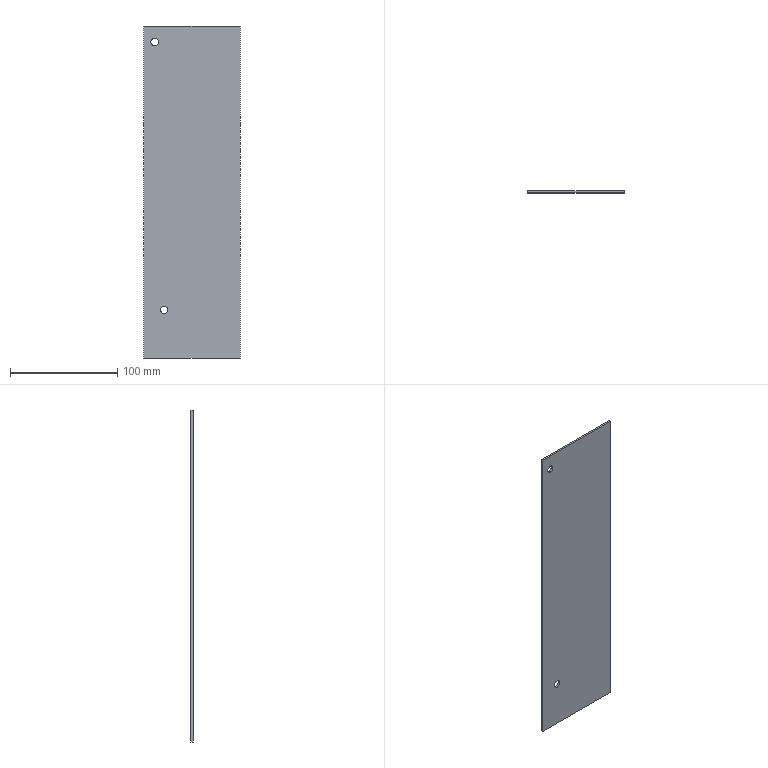Part | STEP file | Bottom plate secondary wiring hole cover | 1 solid | 10 faces | box 90 x 2 x 310 mm | volume 55646 mm3 | plane 6 | cylinder 4 | commonest cylinder face diameters 7 x4
STEP:
#1=CARTESIAN_POINT('',(0.,0.,0.));
#2=DIRECTION('',(0.,0.,1.));
#3=DIRECTION('',(1.,0.,0.));
#4=AXIS2_PLACEMENT_3D('',#1,#2,#3);
#5=CARTESIAN_POINT('',(10.,-2.,-11.5));
#6=VERTEX_POINT('',#5);
#7=CARTESIAN_POINT('',(10.,0.,-11.5));
#8=VERTEX_POINT('',#7);
#9=CARTESIAN_POINT('',(10.,-10.,-11.5));
#10=DIRECTION('',(0.,1.,0.));
#11=VECTOR('',#10,1.);
#12=LINE('',#9,#11);
#13=CARTESIAN_POINT('',(10.,-10.,-15.));
#14=DIRECTION('',(0.,1.,0.));
#15=DIRECTION('',(0.,0.,1.));
#16=AXIS2_PLACEMENT_3D('',#13,#14,#15);
#17=CYLINDRICAL_SURFACE('',#16,3.5);
#18=CARTESIAN_POINT('',(6.283,0.));
#19=DIRECTION('',(0.,1.));
#20=VECTOR('',#19,1.);
#21=LINE('',#18,#20);
#22=(GEOMETRIC_REPRESENTATION_CONTEXT(2)PARAMETRIC_REPRESENTATION_CONTEXT()REPRESENTATION_CONTEXT('',''));
#23=DEFINITIONAL_REPRESENTATION('',(#21),#22);
#24=PCURVE('',#17,#23);
#25=CARTESIAN_POINT('',(10.,-10.,-15.));
#26=DIRECTION('',(0.,1.,0.));
#27=DIRECTION('',(0.,0.,1.));
#28=AXIS2_PLACEMENT_3D('',#25,#26,#27);
#29=CYLINDRICAL_SURFACE('',#28,3.5);
#30=CARTESIAN_POINT('',(0.,0.));
#31=DIRECTION('',(0.,1.));
#32=VECTOR('',#31,1.);
#33=LINE('',#30,#32);
#34=(GEOMETRIC_REPRESENTATION_CONTEXT(2)PARAMETRIC_REPRESENTATION_CONTEXT()REPRESENTATION_CONTEXT('',''));
#35=DEFINITIONAL_REPRESENTATION('',(#33),#34);
#36=PCURVE('',#29,#35);
#37=SURFACE_CURVE('',#12,(#24,#36),.PCURVE_S1.);
#38=EDGE_CURVE('',#6,#8,#37,.T.);
#39=ORIENTED_EDGE('',*,*,#38,.T.);
#40=CARTESIAN_POINT('',(10.,0.,-18.5));
#41=VERTEX_POINT('',#40);
#42=CARTESIAN_POINT('',(10.,0.,-15.));
#43=DIRECTION('',(0.,1.,0.));
#44=DIRECTION('',(0.,0.,1.));
#45=AXIS2_PLACEMENT_3D('',#42,#43,#44);
#46=CIRCLE('',#45,3.5);
#47=CARTESIAN_POINT('',(0.,10.));
#48=DIRECTION('',(1.,0.));
#49=VECTOR('',#48,1.);
#50=LINE('',#47,#49);
#51=(GEOMETRIC_REPRESENTATION_CONTEXT(2)PARAMETRIC_REPRESENTATION_CONTEXT()REPRESENTATION_CONTEXT('',''));
#52=DEFINITIONAL_REPRESENTATION('',(#50),#51);
#53=PCURVE('',#17,#52);
#54=CARTESIAN_POINT('',(0.,0.,0.));
#55=DIRECTION('',(0.,1.,0.));
#56=DIRECTION('',(0.,0.,1.));
#57=AXIS2_PLACEMENT_3D('',#54,#55,#56);
#58=PLANE('',#57);
#59=CARTESIAN_POINT('',(-15.,10.));
#60=DIRECTION('',(1.,0.));
#61=AXIS2_PLACEMENT_2D('',#59,#60);
#62=CIRCLE('',#61,3.5);
#63=(GEOMETRIC_REPRESENTATION_CONTEXT(2)PARAMETRIC_REPRESENTATION_CONTEXT()REPRESENTATION_CONTEXT('',''));
#64=DEFINITIONAL_REPRESENTATION('',(#62),#63);
#65=PCURVE('',#58,#64);
#66=SURFACE_CURVE('',#46,(#53,#65),.PCURVE_S1.);
#67=EDGE_CURVE('',#41,#8,#66,.T.);
#68=ORIENTED_EDGE('',*,*,#67,.F.);
#69=CARTESIAN_POINT('',(10.,-2.,-18.5));
#70=VERTEX_POINT('',#69);
#71=CARTESIAN_POINT('',(10.,-10.,-18.5));
#72=DIRECTION('',(0.,1.,0.));
#73=VECTOR('',#72,1.);
#74=LINE('',#71,#73);
#75=CARTESIAN_POINT('',(3.142,0.));
#76=DIRECTION('',(0.,1.));
#77=VECTOR('',#76,1.);
#78=LINE('',#75,#77);
#79=(GEOMETRIC_REPRESENTATION_CONTEXT(2)PARAMETRIC_REPRESENTATION_CONTEXT()REPRESENTATION_CONTEXT('',''));
#80=DEFINITIONAL_REPRESENTATION('',(#78),#79);
#81=PCURVE('',#17,#80);
#82=CARTESIAN_POINT('',(3.142,0.));
#83=DIRECTION('',(0.,1.));
#84=VECTOR('',#83,1.);
#85=LINE('',#82,#84);
#86=(GEOMETRIC_REPRESENTATION_CONTEXT(2)PARAMETRIC_REPRESENTATION_CONTEXT()REPRESENTATION_CONTEXT('',''));
#87=DEFINITIONAL_REPRESENTATION('',(#85),#86);
#88=PCURVE('',#29,#87);
#89=SURFACE_CURVE('',#74,(#81,#88),.PCURVE_S1.);
#90=EDGE_CURVE('',#70,#41,#89,.T.);
#91=ORIENTED_EDGE('',*,*,#90,.F.);
#92=CARTESIAN_POINT('',(10.,-2.,-15.));
#93=DIRECTION('',(0.,1.,0.));
#94=DIRECTION('',(0.,0.,1.));
#95=AXIS2_PLACEMENT_3D('',#92,#93,#94);
#96=CIRCLE('',#95,3.5);
#97=CARTESIAN_POINT('',(0.,8.));
#98=DIRECTION('',(1.,0.));
#99=VECTOR('',#98,1.);
#100=LINE('',#97,#99);
#101=(GEOMETRIC_REPRESENTATION_CONTEXT(2)PARAMETRIC_REPRESENTATION_CONTEXT()REPRESENTATION_CONTEXT('',''));
#102=DEFINITIONAL_REPRESENTATION('',(#100),#101);
#103=PCURVE('',#17,#102);
#104=CARTESIAN_POINT('',(0.,-2.,0.));
#105=DIRECTION('',(0.,1.,0.));
#106=DIRECTION('',(0.,0.,1.));
#107=AXIS2_PLACEMENT_3D('',#104,#105,#106);
#108=PLANE('',#107);
#109=CARTESIAN_POINT('',(-15.,10.));
#110=DIRECTION('',(1.,0.));
#111=AXIS2_PLACEMENT_2D('',#109,#110);
#112=CIRCLE('',#111,3.5);
#113=(GEOMETRIC_REPRESENTATION_CONTEXT(2)PARAMETRIC_REPRESENTATION_CONTEXT()REPRESENTATION_CONTEXT('',''));
#114=DEFINITIONAL_REPRESENTATION('',(#112),#113);
#115=PCURVE('',#108,#114);
#116=SURFACE_CURVE('',#96,(#103,#115),.PCURVE_S1.);
#117=EDGE_CURVE('',#70,#6,#116,.T.);
#118=ORIENTED_EDGE('',*,*,#117,.T.);
#119=EDGE_LOOP('',(#39,#68,#91,#118));
#120=FACE_BOUND('',#119,.F.);
#121=ADVANCED_FACE('',(#120),#17,.F.);
#122=CARTESIAN_POINT('',(19.,-2.,-261.5));
#123=VERTEX_POINT('',#122);
#124=CARTESIAN_POINT('',(19.,0.,-261.5));
#125=VERTEX_POINT('',#124);
#126=CARTESIAN_POINT('',(19.,-10.,-261.5));
#127=DIRECTION('',(0.,1.,0.));
#128=VECTOR('',#127,1.);
#129=LINE('',#126,#128);
#130=CARTESIAN_POINT('',(19.,-10.,-265.));
#131=DIRECTION('',(0.,1.,0.));
#132=DIRECTION('',(0.,0.,1.));
#133=AXIS2_PLACEMENT_3D('',#130,#131,#132);
#134=CYLINDRICAL_SURFACE('',#133,3.5);
#135=CARTESIAN_POINT('',(6.283,0.));
#136=DIRECTION('',(0.,1.));
#137=VECTOR('',#136,1.);
#138=LINE('',#135,#137);
#139=(GEOMETRIC_REPRESENTATION_CONTEXT(2)PARAMETRIC_REPRESENTATION_CONTEXT()REPRESENTATION_CONTEXT('',''));
#140=DEFINITIONAL_REPRESENTATION('',(#138),#139);
#141=PCURVE('',#134,#140);
#142=CARTESIAN_POINT('',(19.,-10.,-265.));
#143=DIRECTION('',(0.,1.,0.));
#144=DIRECTION('',(0.,0.,1.));
#145=AXIS2_PLACEMENT_3D('',#142,#143,#144);
#146=CYLINDRICAL_SURFACE('',#145,3.5);
#147=CARTESIAN_POINT('',(0.,0.));
#148=DIRECTION('',(0.,1.));
#149=VECTOR('',#148,1.);
#150=LINE('',#147,#149);
#151=(GEOMETRIC_REPRESENTATION_CONTEXT(2)PARAMETRIC_REPRESENTATION_CONTEXT()REPRESENTATION_CONTEXT('',''));
#152=DEFINITIONAL_REPRESENTATION('',(#150),#151);
#153=PCURVE('',#146,#152);
#154=SURFACE_CURVE('',#129,(#141,#153),.PCURVE_S1.);
#155=EDGE_CURVE('',#123,#125,#154,.T.);
#156=ORIENTED_EDGE('',*,*,#155,.T.);
#157=CARTESIAN_POINT('',(19.,0.,-268.5));
#158=VERTEX_POINT('',#157);
#159=CARTESIAN_POINT('',(19.,0.,-265.));
#160=DIRECTION('',(0.,1.,0.));
#161=DIRECTION('',(0.,0.,1.));
#162=AXIS2_PLACEMENT_3D('',#159,#160,#161);
#163=CIRCLE('',#162,3.5);
#164=CARTESIAN_POINT('',(0.,10.));
#165=DIRECTION('',(1.,0.));
#166=VECTOR('',#165,1.);
#167=LINE('',#164,#166);
#168=(GEOMETRIC_REPRESENTATION_CONTEXT(2)PARAMETRIC_REPRESENTATION_CONTEXT()REPRESENTATION_CONTEXT('',''));
#169=DEFINITIONAL_REPRESENTATION('',(#167),#168);
#170=PCURVE('',#134,#169);
#171=CARTESIAN_POINT('',(-265.,19.));
#172=DIRECTION('',(1.,0.));
#173=AXIS2_PLACEMENT_2D('',#171,#172);
#174=CIRCLE('',#173,3.5);
#175=(GEOMETRIC_REPRESENTATION_CONTEXT(2)PARAMETRIC_REPRESENTATION_CONTEXT()REPRESENTATION_CONTEXT('',''));
#176=DEFINITIONAL_REPRESENTATION('',(#174),#175);
#177=PCURVE('',#58,#176);
#178=SURFACE_CURVE('',#163,(#170,#177),.PCURVE_S1.);
#179=EDGE_CURVE('',#158,#125,#178,.T.);
#180=ORIENTED_EDGE('',*,*,#179,.F.);
#181=CARTESIAN_POINT('',(19.,-2.,-268.5));
#182=VERTEX_POINT('',#181);
#183=CARTESIAN_POINT('',(19.,-10.,-268.5));
#184=DIRECTION('',(0.,1.,0.));
#185=VECTOR('',#184,1.);
#186=LINE('',#183,#185);
#187=CARTESIAN_POINT('',(3.142,0.));
#188=DIRECTION('',(0.,1.));
#189=VECTOR('',#188,1.);
#190=LINE('',#187,#189);
#191=(GEOMETRIC_REPRESENTATION_CONTEXT(2)PARAMETRIC_REPRESENTATION_CONTEXT()REPRESENTATION_CONTEXT('',''));
#192=DEFINITIONAL_REPRESENTATION('',(#190),#191);
#193=PCURVE('',#134,#192);
#194=CARTESIAN_POINT('',(3.142,0.));
#195=DIRECTION('',(0.,1.));
#196=VECTOR('',#195,1.);
#197=LINE('',#194,#196);
#198=(GEOMETRIC_REPRESENTATION_CONTEXT(2)PARAMETRIC_REPRESENTATION_CONTEXT()REPRESENTATION_CONTEXT('',''));
#199=DEFINITIONAL_REPRESENTATION('',(#197),#198);
#200=PCURVE('',#146,#199);
#201=SURFACE_CURVE('',#186,(#193,#200),.PCURVE_S1.);
#202=EDGE_CURVE('',#182,#158,#201,.T.);
#203=ORIENTED_EDGE('',*,*,#202,.F.);
#204=CARTESIAN_POINT('',(19.,-2.,-265.));
#205=DIRECTION('',(0.,1.,0.));
#206=DIRECTION('',(0.,0.,1.));
#207=AXIS2_PLACEMENT_3D('',#204,#205,#206);
#208=CIRCLE('',#207,3.5);
#209=CARTESIAN_POINT('',(0.,8.));
#210=DIRECTION('',(1.,0.));
#211=VECTOR('',#210,1.);
#212=LINE('',#209,#211);
#213=(GEOMETRIC_REPRESENTATION_CONTEXT(2)PARAMETRIC_REPRESENTATION_CONTEXT()REPRESENTATION_CONTEXT('',''));
#214=DEFINITIONAL_REPRESENTATION('',(#212),#213);
#215=PCURVE('',#134,#214);
#216=CARTESIAN_POINT('',(-265.,19.));
#217=DIRECTION('',(1.,0.));
#218=AXIS2_PLACEMENT_2D('',#216,#217);
#219=CIRCLE('',#218,3.5);
#220=(GEOMETRIC_REPRESENTATION_CONTEXT(2)PARAMETRIC_REPRESENTATION_CONTEXT()REPRESENTATION_CONTEXT('',''));
#221=DEFINITIONAL_REPRESENTATION('',(#219),#220);
#222=PCURVE('',#108,#221);
#223=SURFACE_CURVE('',#208,(#215,#222),.PCURVE_S1.);
#224=EDGE_CURVE('',#182,#123,#223,.T.);
#225=ORIENTED_EDGE('',*,*,#224,.T.);
#226=EDGE_LOOP('',(#156,#180,#203,#225));
#227=FACE_BOUND('',#226,.F.);
#228=ADVANCED_FACE('',(#227),#134,.F.);
#229=CARTESIAN_POINT('',(0.,0.,-310.));
#230=VERTEX_POINT('',#229);
#231=CARTESIAN_POINT('',(0.,0.,0.));
#232=VERTEX_POINT('',#231);
#233=CARTESIAN_POINT('',(0.,0.,-310.));
#234=DIRECTION('',(0.,0.,1.));
#235=VECTOR('',#234,1.);
#236=LINE('',#233,#235);
#237=CARTESIAN_POINT('',(0.,-2.,-310.));
#238=DIRECTION('',(-1.,0.,0.));
#239=DIRECTION('',(0.,0.,1.));
#240=AXIS2_PLACEMENT_3D('',#237,#238,#239);
#241=PLANE('',#240);
#242=CARTESIAN_POINT('',(0.,2.));
#243=DIRECTION('',(1.,0.));
#244=VECTOR('',#243,1.);
#245=LINE('',#242,#244);
#246=(GEOMETRIC_REPRESENTATION_CONTEXT(2)PARAMETRIC_REPRESENTATION_CONTEXT()REPRESENTATION_CONTEXT('',''));
#247=DEFINITIONAL_REPRESENTATION('',(#245),#246);
#248=PCURVE('',#241,#247);
#249=CARTESIAN_POINT('',(-310.,0.));
#250=DIRECTION('',(1.,0.));
#251=VECTOR('',#250,1.);
#252=LINE('',#249,#251);
#253=(GEOMETRIC_REPRESENTATION_CONTEXT(2)PARAMETRIC_REPRESENTATION_CONTEXT()REPRESENTATION_CONTEXT('',''));
#254=DEFINITIONAL_REPRESENTATION('',(#252),#253);
#255=PCURVE('',#58,#254);
#256=SURFACE_CURVE('',#236,(#248,#255),.PCURVE_S1.);
#257=EDGE_CURVE('',#230,#232,#256,.T.);
#258=ORIENTED_EDGE('',*,*,#257,.F.);
#259=CARTESIAN_POINT('',(0.,-2.,-310.));
#260=VERTEX_POINT('',#259);
#261=CARTESIAN_POINT('',(0.,-2.,-310.));
#262=DIRECTION('',(0.,1.,0.));
#263=VECTOR('',#262,1.);
#264=LINE('',#261,#263);
#265=CARTESIAN_POINT('',(0.,0.));
#266=DIRECTION('',(0.,1.));
#267=VECTOR('',#266,1.);
#268=LINE('',#265,#267);
#269=(GEOMETRIC_REPRESENTATION_CONTEXT(2)PARAMETRIC_REPRESENTATION_CONTEXT()REPRESENTATION_CONTEXT('',''));
#270=DEFINITIONAL_REPRESENTATION('',(#268),#269);
#271=PCURVE('',#241,#270);
#272=CARTESIAN_POINT('',(0.,-2.,-310.));
#273=DIRECTION('',(0.,0.,-1.));
#274=DIRECTION('',(-1.,0.,0.));
#275=AXIS2_PLACEMENT_3D('',#272,#273,#274);
#276=PLANE('',#275);
#277=CARTESIAN_POINT('',(0.,0.));
#278=DIRECTION('',(0.,1.));
#279=VECTOR('',#278,1.);
#280=LINE('',#277,#279);
#281=(GEOMETRIC_REPRESENTATION_CONTEXT(2)PARAMETRIC_REPRESENTATION_CONTEXT()REPRESENTATION_CONTEXT('',''));
#282=DEFINITIONAL_REPRESENTATION('',(#280),#281);
#283=PCURVE('',#276,#282);
#284=SURFACE_CURVE('',#264,(#271,#283),.PCURVE_S1.);
#285=EDGE_CURVE('',#260,#230,#284,.T.);
#286=ORIENTED_EDGE('',*,*,#285,.F.);
#287=CARTESIAN_POINT('',(0.,-2.,0.));
#288=VERTEX_POINT('',#287);
#289=CARTESIAN_POINT('',(0.,-2.,-310.));
#290=DIRECTION('',(0.,0.,1.));
#291=VECTOR('',#290,1.);
#292=LINE('',#289,#291);
#293=CARTESIAN_POINT('',(0.,0.));
#294=DIRECTION('',(1.,0.));
#295=VECTOR('',#294,1.);
#296=LINE('',#293,#295);
#297=(GEOMETRIC_REPRESENTATION_CONTEXT(2)PARAMETRIC_REPRESENTATION_CONTEXT()REPRESENTATION_CONTEXT('',''));
#298=DEFINITIONAL_REPRESENTATION('',(#296),#297);
#299=PCURVE('',#241,#298);
#300=CARTESIAN_POINT('',(-310.,0.));
#301=DIRECTION('',(1.,0.));
#302=VECTOR('',#301,1.);
#303=LINE('',#300,#302);
#304=(GEOMETRIC_REPRESENTATION_CONTEXT(2)PARAMETRIC_REPRESENTATION_CONTEXT()REPRESENTATION_CONTEXT('',''));
#305=DEFINITIONAL_REPRESENTATION('',(#303),#304);
#306=PCURVE('',#108,#305);
#307=SURFACE_CURVE('',#292,(#299,#306),.PCURVE_S1.);
#308=EDGE_CURVE('',#260,#288,#307,.T.);
#309=ORIENTED_EDGE('',*,*,#308,.T.);
#310=CARTESIAN_POINT('',(0.,-2.,0.));
#311=DIRECTION('',(0.,1.,0.));
#312=VECTOR('',#311,1.);
#313=LINE('',#310,#312);
#314=CARTESIAN_POINT('',(310.,0.));
#315=DIRECTION('',(0.,1.));
#316=VECTOR('',#315,1.);
#317=LINE('',#314,#316);
#318=(GEOMETRIC_REPRESENTATION_CONTEXT(2)PARAMETRIC_REPRESENTATION_CONTEXT()REPRESENTATION_CONTEXT('',''));
#319=DEFINITIONAL_REPRESENTATION('',(#317),#318);
#320=PCURVE('',#241,#319);
#321=CARTESIAN_POINT('',(0.,-2.,0.));
#322=DIRECTION('',(0.,0.,1.));
#323=DIRECTION('',(1.,0.,0.));
#324=AXIS2_PLACEMENT_3D('',#321,#322,#323);
#325=PLANE('',#324);
#326=CARTESIAN_POINT('',(0.,0.));
#327=DIRECTION('',(0.,1.));
#328=VECTOR('',#327,1.);
#329=LINE('',#326,#328);
#330=(GEOMETRIC_REPRESENTATION_CONTEXT(2)PARAMETRIC_REPRESENTATION_CONTEXT()REPRESENTATION_CONTEXT('',''));
#331=DEFINITIONAL_REPRESENTATION('',(#329),#330);
#332=PCURVE('',#325,#331);
#333=SURFACE_CURVE('',#313,(#320,#332),.PCURVE_S1.);
#334=EDGE_CURVE('',#288,#232,#333,.T.);
#335=ORIENTED_EDGE('',*,*,#334,.T.);
#336=EDGE_LOOP('',(#258,#286,#309,#335));
#337=FACE_BOUND('',#336,.T.);
#338=ADVANCED_FACE('',(#337),#241,.T.);
#339=CARTESIAN_POINT('',(90.,0.,-310.));
#340=VERTEX_POINT('',#339);
#341=CARTESIAN_POINT('',(0.,0.,-310.));
#342=DIRECTION('',(-1.,0.,0.));
#343=VECTOR('',#342,1.);
#344=LINE('',#341,#343);
#345=CARTESIAN_POINT('',(0.,2.));
#346=DIRECTION('',(1.,0.));
#347=VECTOR('',#346,1.);
#348=LINE('',#345,#347);
#349=(GEOMETRIC_REPRESENTATION_CONTEXT(2)PARAMETRIC_REPRESENTATION_CONTEXT()REPRESENTATION_CONTEXT('',''));
#350=DEFINITIONAL_REPRESENTATION('',(#348),#349);
#351=PCURVE('',#276,#350);
#352=CARTESIAN_POINT('',(-310.,0.));
#353=DIRECTION('',(0.,-1.));
#354=VECTOR('',#353,1.);
#355=LINE('',#352,#354);
#356=(GEOMETRIC_REPRESENTATION_CONTEXT(2)PARAMETRIC_REPRESENTATION_CONTEXT()REPRESENTATION_CONTEXT('',''));
#357=DEFINITIONAL_REPRESENTATION('',(#355),#356);
#358=PCURVE('',#58,#357);
#359=SURFACE_CURVE('',#344,(#351,#358),.PCURVE_S1.);
#360=EDGE_CURVE('',#340,#230,#359,.T.);
#361=ORIENTED_EDGE('',*,*,#360,.F.);
#362=CARTESIAN_POINT('',(90.,-2.,-310.));
#363=VERTEX_POINT('',#362);
#364=CARTESIAN_POINT('',(90.,-2.,-310.));
#365=DIRECTION('',(0.,1.,0.));
#366=VECTOR('',#365,1.);
#367=LINE('',#364,#366);
#368=CARTESIAN_POINT('',(-90.,0.));
#369=DIRECTION('',(0.,1.));
#370=VECTOR('',#369,1.);
#371=LINE('',#368,#370);
#372=(GEOMETRIC_REPRESENTATION_CONTEXT(2)PARAMETRIC_REPRESENTATION_CONTEXT()REPRESENTATION_CONTEXT('',''));
#373=DEFINITIONAL_REPRESENTATION('',(#371),#372);
#374=PCURVE('',#276,#373);
#375=CARTESIAN_POINT('',(90.,-2.,-310.));
#376=DIRECTION('',(1.,0.,0.));
#377=DIRECTION('',(0.,0.,-1.));
#378=AXIS2_PLACEMENT_3D('',#375,#376,#377);
#379=PLANE('',#378);
#380=CARTESIAN_POINT('',(0.,0.));
#381=DIRECTION('',(0.,1.));
#382=VECTOR('',#381,1.);
#383=LINE('',#380,#382);
#384=(GEOMETRIC_REPRESENTATION_CONTEXT(2)PARAMETRIC_REPRESENTATION_CONTEXT()REPRESENTATION_CONTEXT('',''));
#385=DEFINITIONAL_REPRESENTATION('',(#383),#384);
#386=PCURVE('',#379,#385);
#387=SURFACE_CURVE('',#367,(#374,#386),.PCURVE_S1.);
#388=EDGE_CURVE('',#363,#340,#387,.T.);
#389=ORIENTED_EDGE('',*,*,#388,.F.);
#390=CARTESIAN_POINT('',(0.,-2.,-310.));
#391=DIRECTION('',(-1.,0.,0.));
#392=VECTOR('',#391,1.);
#393=LINE('',#390,#392);
#394=CARTESIAN_POINT('',(0.,0.));
#395=DIRECTION('',(1.,0.));
#396=VECTOR('',#395,1.);
#397=LINE('',#394,#396);
#398=(GEOMETRIC_REPRESENTATION_CONTEXT(2)PARAMETRIC_REPRESENTATION_CONTEXT()REPRESENTATION_CONTEXT('',''));
#399=DEFINITIONAL_REPRESENTATION('',(#397),#398);
#400=PCURVE('',#276,#399);
#401=CARTESIAN_POINT('',(-310.,0.));
#402=DIRECTION('',(0.,-1.));
#403=VECTOR('',#402,1.);
#404=LINE('',#401,#403);
#405=(GEOMETRIC_REPRESENTATION_CONTEXT(2)PARAMETRIC_REPRESENTATION_CONTEXT()REPRESENTATION_CONTEXT('',''));
#406=DEFINITIONAL_REPRESENTATION('',(#404),#405);
#407=PCURVE('',#108,#406);
#408=SURFACE_CURVE('',#393,(#400,#407),.PCURVE_S1.);
#409=EDGE_CURVE('',#363,#260,#408,.T.);
#410=ORIENTED_EDGE('',*,*,#409,.T.);
#411=ORIENTED_EDGE('',*,*,#285,.T.);
#412=EDGE_LOOP('',(#361,#389,#410,#411));
#413=FACE_BOUND('',#412,.T.);
#414=ADVANCED_FACE('',(#413),#276,.T.);
#415=CARTESIAN_POINT('',(90.,0.,0.));
#416=VERTEX_POINT('',#415);
#417=CARTESIAN_POINT('',(90.,0.,-310.));
#418=DIRECTION('',(0.,0.,-1.));
#419=VECTOR('',#418,1.);
#420=LINE('',#417,#419);
#421=CARTESIAN_POINT('',(0.,2.));
#422=DIRECTION('',(1.,0.));
#423=VECTOR('',#422,1.);
#424=LINE('',#421,#423);
#425=(GEOMETRIC_REPRESENTATION_CONTEXT(2)PARAMETRIC_REPRESENTATION_CONTEXT()REPRESENTATION_CONTEXT('',''));
#426=DEFINITIONAL_REPRESENTATION('',(#424),#425);
#427=PCURVE('',#379,#426);
#428=CARTESIAN_POINT('',(-310.,90.));
#429=DIRECTION('',(-1.,0.));
#430=VECTOR('',#429,1.);
#431=LINE('',#428,#430);
#432=(GEOMETRIC_REPRESENTATION_CONTEXT(2)PARAMETRIC_REPRESENTATION_CONTEXT()REPRESENTATION_CONTEXT('',''));
#433=DEFINITIONAL_REPRESENTATION('',(#431),#432);
#434=PCURVE('',#58,#433);
#435=SURFACE_CURVE('',#420,(#427,#434),.PCURVE_S1.);
#436=EDGE_CURVE('',#416,#340,#435,.T.);
#437=ORIENTED_EDGE('',*,*,#436,.F.);
#438=CARTESIAN_POINT('',(90.,-2.,0.));
#439=VERTEX_POINT('',#438);
#440=CARTESIAN_POINT('',(90.,-2.,0.));
#441=DIRECTION('',(0.,1.,0.));
#442=VECTOR('',#441,1.);
#443=LINE('',#440,#442);
#444=CARTESIAN_POINT('',(-310.,0.));
#445=DIRECTION('',(0.,1.));
#446=VECTOR('',#445,1.);
#447=LINE('',#444,#446);
#448=(GEOMETRIC_REPRESENTATION_CONTEXT(2)PARAMETRIC_REPRESENTATION_CONTEXT()REPRESENTATION_CONTEXT('',''));
#449=DEFINITIONAL_REPRESENTATION('',(#447),#448);
#450=PCURVE('',#379,#449);
#451=CARTESIAN_POINT('',(90.,0.));
#452=DIRECTION('',(0.,1.));
#453=VECTOR('',#452,1.);
#454=LINE('',#451,#453);
#455=(GEOMETRIC_REPRESENTATION_CONTEXT(2)PARAMETRIC_REPRESENTATION_CONTEXT()REPRESENTATION_CONTEXT('',''));
#456=DEFINITIONAL_REPRESENTATION('',(#454),#455);
#457=PCURVE('',#325,#456);
#458=SURFACE_CURVE('',#443,(#450,#457),.PCURVE_S1.);
#459=EDGE_CURVE('',#439,#416,#458,.T.);
#460=ORIENTED_EDGE('',*,*,#459,.F.);
#461=CARTESIAN_POINT('',(90.,-2.,-310.));
#462=DIRECTION('',(0.,0.,-1.));
#463=VECTOR('',#462,1.);
#464=LINE('',#461,#463);
#465=CARTESIAN_POINT('',(0.,0.));
#466=DIRECTION('',(1.,0.));
#467=VECTOR('',#466,1.);
#468=LINE('',#465,#467);
#469=(GEOMETRIC_REPRESENTATION_CONTEXT(2)PARAMETRIC_REPRESENTATION_CONTEXT()REPRESENTATION_CONTEXT('',''));
#470=DEFINITIONAL_REPRESENTATION('',(#468),#469);
#471=PCURVE('',#379,#470);
#472=CARTESIAN_POINT('',(-310.,90.));
#473=DIRECTION('',(-1.,0.));
#474=VECTOR('',#473,1.);
#475=LINE('',#472,#474);
#476=(GEOMETRIC_REPRESENTATION_CONTEXT(2)PARAMETRIC_REPRESENTATION_CONTEXT()REPRESENTATION_CONTEXT('',''));
#477=DEFINITIONAL_REPRESENTATION('',(#475),#476);
#478=PCURVE('',#108,#477);
#479=SURFACE_CURVE('',#464,(#471,#478),.PCURVE_S1.);
#480=EDGE_CURVE('',#439,#363,#479,.T.);
#481=ORIENTED_EDGE('',*,*,#480,.T.);
#482=ORIENTED_EDGE('',*,*,#388,.T.);
#483=EDGE_LOOP('',(#437,#460,#481,#482));
#484=FACE_BOUND('',#483,.T.);
#485=ADVANCED_FACE('',(#484),#379,.T.);
#486=CARTESIAN_POINT('',(0.,0.,0.));
#487=DIRECTION('',(1.,0.,0.));
#488=VECTOR('',#487,1.);
#489=LINE('',#486,#488);
#490=CARTESIAN_POINT('',(0.,2.));
#491=DIRECTION('',(1.,0.));
#492=VECTOR('',#491,1.);
#493=LINE('',#490,#492);
#494=(GEOMETRIC_REPRESENTATION_CONTEXT(2)PARAMETRIC_REPRESENTATION_CONTEXT()REPRESENTATION_CONTEXT('',''));
#495=DEFINITIONAL_REPRESENTATION('',(#493),#494);
#496=PCURVE('',#325,#495);
#497=CARTESIAN_POINT('',(0.,0.));
#498=DIRECTION('',(0.,1.));
#499=VECTOR('',#498,1.);
#500=LINE('',#497,#499);
#501=(GEOMETRIC_REPRESENTATION_CONTEXT(2)PARAMETRIC_REPRESENTATION_CONTEXT()REPRESENTATION_CONTEXT('',''));
#502=DEFINITIONAL_REPRESENTATION('',(#500),#501);
#503=PCURVE('',#58,#502);
#504=SURFACE_CURVE('',#489,(#496,#503),.PCURVE_S1.);
#505=EDGE_CURVE('',#232,#416,#504,.T.);
#506=ORIENTED_EDGE('',*,*,#505,.F.);
#507=ORIENTED_EDGE('',*,*,#334,.F.);
#508=CARTESIAN_POINT('',(0.,-2.,0.));
#509=DIRECTION('',(1.,0.,0.));
#510=VECTOR('',#509,1.);
#511=LINE('',#508,#510);
#512=CARTESIAN_POINT('',(0.,0.));
#513=DIRECTION('',(1.,0.));
#514=VECTOR('',#513,1.);
#515=LINE('',#512,#514);
#516=(GEOMETRIC_REPRESENTATION_CONTEXT(2)PARAMETRIC_REPRESENTATION_CONTEXT()REPRESENTATION_CONTEXT('',''));
#517=DEFINITIONAL_REPRESENTATION('',(#515),#516);
#518=PCURVE('',#325,#517);
#519=CARTESIAN_POINT('',(0.,0.));
#520=DIRECTION('',(0.,1.));
#521=VECTOR('',#520,1.);
#522=LINE('',#519,#521);
#523=(GEOMETRIC_REPRESENTATION_CONTEXT(2)PARAMETRIC_REPRESENTATION_CONTEXT()REPRESENTATION_CONTEXT('',''));
#524=DEFINITIONAL_REPRESENTATION('',(#522),#523);
#525=PCURVE('',#108,#524);
#526=SURFACE_CURVE('',#511,(#518,#525),.PCURVE_S1.);
#527=EDGE_CURVE('',#288,#439,#526,.T.);
#528=ORIENTED_EDGE('',*,*,#527,.T.);
#529=ORIENTED_EDGE('',*,*,#459,.T.);
#530=EDGE_LOOP('',(#506,#507,#528,#529));
#531=FACE_BOUND('',#530,.T.);
#532=ADVANCED_FACE('',(#531),#325,.T.);
#533=CARTESIAN_POINT('',(10.,-2.,-15.));
#534=DIRECTION('',(0.,1.,0.));
#535=DIRECTION('',(0.,0.,1.));
#536=AXIS2_PLACEMENT_3D('',#533,#534,#535);
#537=CIRCLE('',#536,3.5);
#538=CARTESIAN_POINT('',(-15.,10.));
#539=DIRECTION('',(1.,0.));
#540=AXIS2_PLACEMENT_2D('',#538,#539);
#541=CIRCLE('',#540,3.5);
#542=(GEOMETRIC_REPRESENTATION_CONTEXT(2)PARAMETRIC_REPRESENTATION_CONTEXT()REPRESENTATION_CONTEXT('',''));
#543=DEFINITIONAL_REPRESENTATION('',(#541),#542);
#544=PCURVE('',#108,#543);
#545=CARTESIAN_POINT('',(0.,8.));
#546=DIRECTION('',(1.,0.));
#547=VECTOR('',#546,1.);
#548=LINE('',#545,#547);
#549=(GEOMETRIC_REPRESENTATION_CONTEXT(2)PARAMETRIC_REPRESENTATION_CONTEXT()REPRESENTATION_CONTEXT('',''));
#550=DEFINITIONAL_REPRESENTATION('',(#548),#549);
#551=PCURVE('',#29,#550);
#552=SURFACE_CURVE('',#537,(#544,#551),.PCURVE_S1.);
#553=EDGE_CURVE('',#6,#70,#552,.T.);
#554=ORIENTED_EDGE('',*,*,#553,.T.);
#555=ORIENTED_EDGE('',*,*,#117,.T.);
#556=EDGE_LOOP('',(#554,#555));
#557=FACE_BOUND('',#556,.T.);
#558=CARTESIAN_POINT('',(19.,-2.,-265.));
#559=DIRECTION('',(0.,1.,0.));
#560=DIRECTION('',(0.,0.,1.));
#561=AXIS2_PLACEMENT_3D('',#558,#559,#560);
#562=CIRCLE('',#561,3.5);
#563=CARTESIAN_POINT('',(-265.,19.));
#564=DIRECTION('',(1.,0.));
#565=AXIS2_PLACEMENT_2D('',#563,#564);
#566=CIRCLE('',#565,3.5);
#567=(GEOMETRIC_REPRESENTATION_CONTEXT(2)PARAMETRIC_REPRESENTATION_CONTEXT()REPRESENTATION_CONTEXT('',''));
#568=DEFINITIONAL_REPRESENTATION('',(#566),#567);
#569=PCURVE('',#108,#568);
#570=CARTESIAN_POINT('',(0.,8.));
#571=DIRECTION('',(1.,0.));
#572=VECTOR('',#571,1.);
#573=LINE('',#570,#572);
#574=(GEOMETRIC_REPRESENTATION_CONTEXT(2)PARAMETRIC_REPRESENTATION_CONTEXT()REPRESENTATION_CONTEXT('',''));
#575=DEFINITIONAL_REPRESENTATION('',(#573),#574);
#576=PCURVE('',#146,#575);
#577=SURFACE_CURVE('',#562,(#569,#576),.PCURVE_S1.);
#578=EDGE_CURVE('',#123,#182,#577,.T.);
#579=ORIENTED_EDGE('',*,*,#578,.T.);
#580=ORIENTED_EDGE('',*,*,#224,.T.);
#581=EDGE_LOOP('',(#579,#580));
#582=FACE_BOUND('',#581,.T.);
#583=ORIENTED_EDGE('',*,*,#308,.F.);
#584=ORIENTED_EDGE('',*,*,#409,.F.);
#585=ORIENTED_EDGE('',*,*,#480,.F.);
#586=ORIENTED_EDGE('',*,*,#527,.F.);
#587=EDGE_LOOP('',(#583,#584,#585,#586));
#588=FACE_BOUND('',#587,.T.);
#589=ADVANCED_FACE('',(#557,#582,#588),#108,.F.);
#590=CARTESIAN_POINT('',(10.,0.,-15.));
#591=DIRECTION('',(0.,1.,0.));
#592=DIRECTION('',(0.,0.,1.));
#593=AXIS2_PLACEMENT_3D('',#590,#591,#592);
#594=CIRCLE('',#593,3.5);
#595=CARTESIAN_POINT('',(-15.,10.));
#596=DIRECTION('',(1.,0.));
#597=AXIS2_PLACEMENT_2D('',#595,#596);
#598=CIRCLE('',#597,3.5);
#599=(GEOMETRIC_REPRESENTATION_CONTEXT(2)PARAMETRIC_REPRESENTATION_CONTEXT()REPRESENTATION_CONTEXT('',''));
#600=DEFINITIONAL_REPRESENTATION('',(#598),#599);
#601=PCURVE('',#58,#600);
#602=CARTESIAN_POINT('',(0.,10.));
#603=DIRECTION('',(1.,0.));
#604=VECTOR('',#603,1.);
#605=LINE('',#602,#604);
#606=(GEOMETRIC_REPRESENTATION_CONTEXT(2)PARAMETRIC_REPRESENTATION_CONTEXT()REPRESENTATION_CONTEXT('',''));
#607=DEFINITIONAL_REPRESENTATION('',(#605),#606);
#608=PCURVE('',#29,#607);
#609=SURFACE_CURVE('',#594,(#601,#608),.PCURVE_S1.);
#610=EDGE_CURVE('',#8,#41,#609,.T.);
#611=ORIENTED_EDGE('',*,*,#610,.F.);
#612=ORIENTED_EDGE('',*,*,#67,.F.);
#613=EDGE_LOOP('',(#611,#612));
#614=FACE_BOUND('',#613,.T.);
#615=CARTESIAN_POINT('',(19.,0.,-265.));
#616=DIRECTION('',(0.,1.,0.));
#617=DIRECTION('',(0.,0.,1.));
#618=AXIS2_PLACEMENT_3D('',#615,#616,#617);
#619=CIRCLE('',#618,3.5);
#620=CARTESIAN_POINT('',(-265.,19.));
#621=DIRECTION('',(1.,0.));
#622=AXIS2_PLACEMENT_2D('',#620,#621);
#623=CIRCLE('',#622,3.5);
#624=(GEOMETRIC_REPRESENTATION_CONTEXT(2)PARAMETRIC_REPRESENTATION_CONTEXT()REPRESENTATION_CONTEXT('',''));
#625=DEFINITIONAL_REPRESENTATION('',(#623),#624);
#626=PCURVE('',#58,#625);
#627=CARTESIAN_POINT('',(0.,10.));
#628=DIRECTION('',(1.,0.));
#629=VECTOR('',#628,1.);
#630=LINE('',#627,#629);
#631=(GEOMETRIC_REPRESENTATION_CONTEXT(2)PARAMETRIC_REPRESENTATION_CONTEXT()REPRESENTATION_CONTEXT('',''));
#632=DEFINITIONAL_REPRESENTATION('',(#630),#631);
#633=PCURVE('',#146,#632);
#634=SURFACE_CURVE('',#619,(#626,#633),.PCURVE_S1.);
#635=EDGE_CURVE('',#125,#158,#634,.T.);
#636=ORIENTED_EDGE('',*,*,#635,.F.);
#637=ORIENTED_EDGE('',*,*,#179,.F.);
#638=EDGE_LOOP('',(#636,#637));
#639=FACE_BOUND('',#638,.T.);
#640=ORIENTED_EDGE('',*,*,#257,.T.);
#641=ORIENTED_EDGE('',*,*,#505,.T.);
#642=ORIENTED_EDGE('',*,*,#436,.T.);
#643=ORIENTED_EDGE('',*,*,#360,.T.);
#644=EDGE_LOOP('',(#640,#641,#642,#643));
#645=FACE_BOUND('',#644,.T.);
#646=ADVANCED_FACE('',(#614,#639,#645),#58,.T.);
#647=ORIENTED_EDGE('',*,*,#635,.F.);
#648=ORIENTED_EDGE('',*,*,#155,.F.);
#649=ORIENTED_EDGE('',*,*,#578,.T.);
#650=ORIENTED_EDGE('',*,*,#202,.T.);
#651=EDGE_LOOP('',(#647,#648,#649,#650));
#652=FACE_BOUND('',#651,.F.);
#653=ADVANCED_FACE('',(#652),#146,.F.);
#654=ORIENTED_EDGE('',*,*,#610,.F.);
#655=ORIENTED_EDGE('',*,*,#38,.F.);
#656=ORIENTED_EDGE('',*,*,#553,.T.);
#657=ORIENTED_EDGE('',*,*,#90,.T.);
#658=EDGE_LOOP('',(#654,#655,#656,#657));
#659=FACE_BOUND('',#658,.F.);
#660=ADVANCED_FACE('',(#659),#29,.F.);
#661=CLOSED_SHELL('',(#121,#228,#338,#414,#485,#532,#589,#646,#653,#660));
#662=MANIFOLD_SOLID_BREP('',#661);
#663=(LENGTH_UNIT()NAMED_UNIT(*)SI_UNIT(.MILLI.,.METRE.));
#664=UNCERTAINTY_MEASURE_WITH_UNIT(LENGTH_MEASURE(0.0000001),#663,'','');
#665=(NAMED_UNIT(*)PLANE_ANGLE_UNIT()SI_UNIT($,.RADIAN.));
#666=(NAMED_UNIT(*)SI_UNIT($,.STERADIAN.)SOLID_ANGLE_UNIT());
#667=(GEOMETRIC_REPRESENTATION_CONTEXT(3)GLOBAL_UNCERTAINTY_ASSIGNED_CONTEXT((#664))GLOBAL_UNIT_ASSIGNED_CONTEXT((#663,#665,#666))REPRESENTATION_CONTEXT('',''));
#668=ADVANCED_BREP_SHAPE_REPRESENTATION('',(#4,#662),#667);